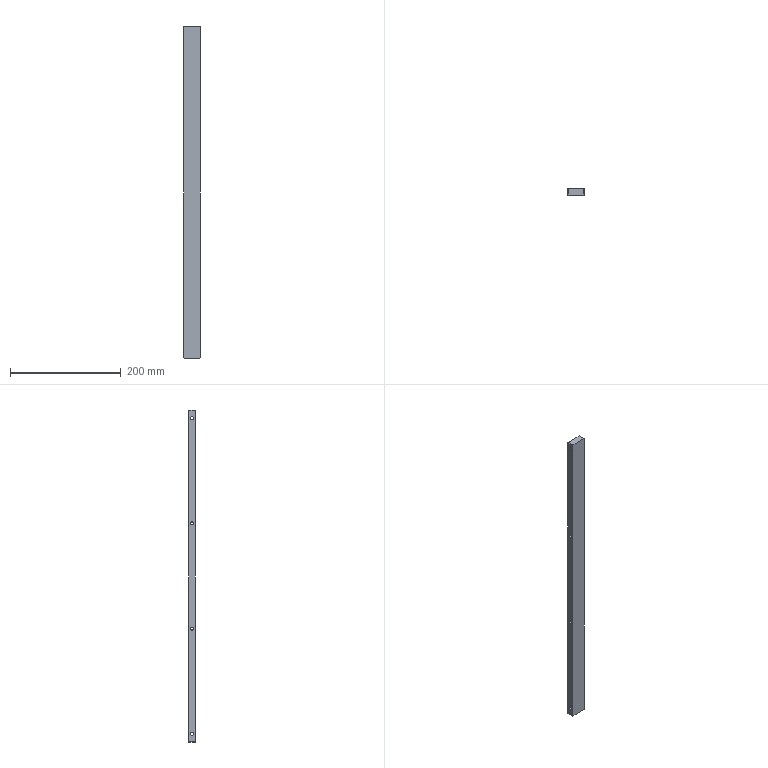Part | NX | features BREP 1 | 1 solid | 30 faces | box 30 x 12 x 600 mm | volume 212029 mm3 | cylinder 16 | plane 14 | commonest cylinder face diameters 5.5 x8 10 x8
STEP:
#1=CARTESIAN_POINT('',(10.,0.,20.));
#2=VERTEX_POINT('',#1);
#3=CARTESIAN_POINT('',(10.,0.,10.));
#4=VERTEX_POINT('',#3);
#5=CARTESIAN_POINT('',(10.,0.,15.));
#6=DIRECTION('',(1.,0.,0.));
#7=DIRECTION('',(0.,0.,-1.));
#8=AXIS2_PLACEMENT_3D('',#5,#6,#7);
#9=CIRCLE('',#8,5.);
#10=EDGE_CURVE('',#2,#4,#9,.T.);
#11=ORIENTED_EDGE('',*,*,#10,.F.);
#12=CARTESIAN_POINT('',(15.,0.,20.));
#13=VERTEX_POINT('',#12);
#14=CARTESIAN_POINT('',(15.,0.,20.));
#15=DIRECTION('',(1.,0.,0.));
#16=VECTOR('',#15,1000.);
#17=LINE('',#14,#16);
#18=EDGE_CURVE('',#2,#13,#17,.T.);
#19=ORIENTED_EDGE('',*,*,#18,.T.);
#20=CARTESIAN_POINT('',(15.,0.,10.));
#21=VERTEX_POINT('',#20);
#22=CARTESIAN_POINT('',(15.,0.,15.));
#23=DIRECTION('',(1.,0.,0.));
#24=DIRECTION('',(0.,0.,-1.));
#25=AXIS2_PLACEMENT_3D('',#22,#23,#24);
#26=CIRCLE('',#25,5.);
#27=EDGE_CURVE('',#13,#21,#26,.T.);
#28=ORIENTED_EDGE('',*,*,#27,.T.);
#29=CARTESIAN_POINT('',(15.,0.,10.));
#30=DIRECTION('',(1.,0.,0.));
#31=VECTOR('',#30,1000.);
#32=LINE('',#29,#31);
#33=EDGE_CURVE('',#4,#21,#32,.T.);
#34=ORIENTED_EDGE('',*,*,#33,.F.);
#35=EDGE_LOOP('',(#11,#19,#28,#34));
#36=FACE_BOUND('',#35,.T.);
#37=CARTESIAN_POINT('',(15.,0.,15.));
#38=DIRECTION('',(1.,0.,0.));
#39=DIRECTION('',(0.,0.,-1.));
#40=AXIS2_PLACEMENT_3D('',#37,#38,#39);
#41=CYLINDRICAL_SURFACE('',#40,5.);
#42=ADVANCED_FACE('',(#36),#41,.F.);
#43=CARTESIAN_POINT('',(-15.,0.,17.75));
#44=VERTEX_POINT('',#43);
#45=CARTESIAN_POINT('',(-15.,0.,12.25));
#46=VERTEX_POINT('',#45);
#47=CARTESIAN_POINT('',(-15.,0.,15.));
#48=DIRECTION('',(1.,0.,0.));
#49=DIRECTION('',(0.,0.,-1.));
#50=AXIS2_PLACEMENT_3D('',#47,#48,#49);
#51=CIRCLE('',#50,2.75);
#52=EDGE_CURVE('',#44,#46,#51,.T.);
#53=ORIENTED_EDGE('',*,*,#52,.F.);
#54=CARTESIAN_POINT('',(10.,0.,17.75));
#55=VERTEX_POINT('',#54);
#56=CARTESIAN_POINT('',(15.,0.,17.75));
#57=DIRECTION('',(1.,0.,0.));
#58=VECTOR('',#57,1000.);
#59=LINE('',#56,#58);
#60=EDGE_CURVE('',#44,#55,#59,.T.);
#61=ORIENTED_EDGE('',*,*,#60,.T.);
#62=CARTESIAN_POINT('',(10.,0.,12.25));
#63=VERTEX_POINT('',#62);
#64=CARTESIAN_POINT('',(10.,0.,15.));
#65=DIRECTION('',(1.,0.,0.));
#66=DIRECTION('',(0.,0.,-1.));
#67=AXIS2_PLACEMENT_3D('',#64,#65,#66);
#68=CIRCLE('',#67,2.75);
#69=EDGE_CURVE('',#55,#63,#68,.T.);
#70=ORIENTED_EDGE('',*,*,#69,.T.);
#71=CARTESIAN_POINT('',(15.,0.,12.25));
#72=DIRECTION('',(1.,0.,0.));
#73=VECTOR('',#72,1000.);
#74=LINE('',#71,#73);
#75=EDGE_CURVE('',#46,#63,#74,.T.);
#76=ORIENTED_EDGE('',*,*,#75,.F.);
#77=EDGE_LOOP('',(#53,#61,#70,#76));
#78=FACE_BOUND('',#77,.T.);
#79=CARTESIAN_POINT('',(15.,0.,15.));
#80=DIRECTION('',(1.,0.,0.));
#81=DIRECTION('',(0.,0.,-1.));
#82=AXIS2_PLACEMENT_3D('',#79,#80,#81);
#83=CYLINDRICAL_SURFACE('',#82,2.75);
#84=ADVANCED_FACE('',(#78),#83,.F.);
#85=CARTESIAN_POINT('',(10.,0.,210.));
#86=VERTEX_POINT('',#85);
#87=CARTESIAN_POINT('',(10.,0.,200.));
#88=VERTEX_POINT('',#87);
#89=CARTESIAN_POINT('',(10.,0.,205.));
#90=DIRECTION('',(1.,0.,0.));
#91=DIRECTION('',(0.,0.,-1.));
#92=AXIS2_PLACEMENT_3D('',#89,#90,#91);
#93=CIRCLE('',#92,5.);
#94=EDGE_CURVE('',#86,#88,#93,.T.);
#95=ORIENTED_EDGE('',*,*,#94,.F.);
#96=CARTESIAN_POINT('',(15.,0.,210.));
#97=VERTEX_POINT('',#96);
#98=CARTESIAN_POINT('',(15.,0.,210.));
#99=DIRECTION('',(1.,0.,0.));
#100=VECTOR('',#99,1000.);
#101=LINE('',#98,#100);
#102=EDGE_CURVE('',#86,#97,#101,.T.);
#103=ORIENTED_EDGE('',*,*,#102,.T.);
#104=CARTESIAN_POINT('',(15.,0.,200.));
#105=VERTEX_POINT('',#104);
#106=CARTESIAN_POINT('',(15.,0.,205.));
#107=DIRECTION('',(1.,0.,0.));
#108=DIRECTION('',(0.,0.,-1.));
#109=AXIS2_PLACEMENT_3D('',#106,#107,#108);
#110=CIRCLE('',#109,5.);
#111=EDGE_CURVE('',#97,#105,#110,.T.);
#112=ORIENTED_EDGE('',*,*,#111,.T.);
#113=CARTESIAN_POINT('',(15.,0.,200.));
#114=DIRECTION('',(1.,0.,0.));
#115=VECTOR('',#114,1000.);
#116=LINE('',#113,#115);
#117=EDGE_CURVE('',#88,#105,#116,.T.);
#118=ORIENTED_EDGE('',*,*,#117,.F.);
#119=EDGE_LOOP('',(#95,#103,#112,#118));
#120=FACE_BOUND('',#119,.T.);
#121=CARTESIAN_POINT('',(15.,0.,205.));
#122=DIRECTION('',(1.,0.,0.));
#123=DIRECTION('',(0.,0.,-1.));
#124=AXIS2_PLACEMENT_3D('',#121,#122,#123);
#125=CYLINDRICAL_SURFACE('',#124,5.);
#126=ADVANCED_FACE('',(#120),#125,.F.);
#127=CARTESIAN_POINT('',(-15.,0.,207.75));
#128=VERTEX_POINT('',#127);
#129=CARTESIAN_POINT('',(-15.,0.,202.25));
#130=VERTEX_POINT('',#129);
#131=CARTESIAN_POINT('',(-15.,0.,205.));
#132=DIRECTION('',(1.,0.,0.));
#133=DIRECTION('',(0.,0.,-1.));
#134=AXIS2_PLACEMENT_3D('',#131,#132,#133);
#135=CIRCLE('',#134,2.75);
#136=EDGE_CURVE('',#128,#130,#135,.T.);
#137=ORIENTED_EDGE('',*,*,#136,.F.);
#138=CARTESIAN_POINT('',(10.,0.,207.75));
#139=VERTEX_POINT('',#138);
#140=CARTESIAN_POINT('',(15.,0.,207.75));
#141=DIRECTION('',(1.,0.,0.));
#142=VECTOR('',#141,1000.);
#143=LINE('',#140,#142);
#144=EDGE_CURVE('',#128,#139,#143,.T.);
#145=ORIENTED_EDGE('',*,*,#144,.T.);
#146=CARTESIAN_POINT('',(10.,0.,202.25));
#147=VERTEX_POINT('',#146);
#148=CARTESIAN_POINT('',(10.,0.,205.));
#149=DIRECTION('',(1.,0.,0.));
#150=DIRECTION('',(0.,0.,-1.));
#151=AXIS2_PLACEMENT_3D('',#148,#149,#150);
#152=CIRCLE('',#151,2.75);
#153=EDGE_CURVE('',#139,#147,#152,.T.);
#154=ORIENTED_EDGE('',*,*,#153,.T.);
#155=CARTESIAN_POINT('',(15.,0.,202.25));
#156=DIRECTION('',(1.,0.,0.));
#157=VECTOR('',#156,1000.);
#158=LINE('',#155,#157);
#159=EDGE_CURVE('',#130,#147,#158,.T.);
#160=ORIENTED_EDGE('',*,*,#159,.F.);
#161=EDGE_LOOP('',(#137,#145,#154,#160));
#162=FACE_BOUND('',#161,.T.);
#163=CARTESIAN_POINT('',(15.,0.,205.));
#164=DIRECTION('',(1.,0.,0.));
#165=DIRECTION('',(0.,0.,-1.));
#166=AXIS2_PLACEMENT_3D('',#163,#164,#165);
#167=CYLINDRICAL_SURFACE('',#166,2.75);
#168=ADVANCED_FACE('',(#162),#167,.F.);
#169=CARTESIAN_POINT('',(10.,0.,400.));
#170=VERTEX_POINT('',#169);
#171=CARTESIAN_POINT('',(10.,0.,390.));
#172=VERTEX_POINT('',#171);
#173=CARTESIAN_POINT('',(10.,0.,395.));
#174=DIRECTION('',(1.,0.,0.));
#175=DIRECTION('',(0.,0.,-1.));
#176=AXIS2_PLACEMENT_3D('',#173,#174,#175);
#177=CIRCLE('',#176,5.);
#178=EDGE_CURVE('',#170,#172,#177,.T.);
#179=ORIENTED_EDGE('',*,*,#178,.F.);
#180=CARTESIAN_POINT('',(15.,0.,400.));
#181=VERTEX_POINT('',#180);
#182=CARTESIAN_POINT('',(15.,0.,400.));
#183=DIRECTION('',(1.,0.,0.));
#184=VECTOR('',#183,1000.);
#185=LINE('',#182,#184);
#186=EDGE_CURVE('',#170,#181,#185,.T.);
#187=ORIENTED_EDGE('',*,*,#186,.T.);
#188=CARTESIAN_POINT('',(15.,0.,390.));
#189=VERTEX_POINT('',#188);
#190=CARTESIAN_POINT('',(15.,0.,395.));
#191=DIRECTION('',(1.,0.,0.));
#192=DIRECTION('',(0.,0.,-1.));
#193=AXIS2_PLACEMENT_3D('',#190,#191,#192);
#194=CIRCLE('',#193,5.);
#195=EDGE_CURVE('',#181,#189,#194,.T.);
#196=ORIENTED_EDGE('',*,*,#195,.T.);
#197=CARTESIAN_POINT('',(15.,0.,390.));
#198=DIRECTION('',(1.,0.,0.));
#199=VECTOR('',#198,1000.);
#200=LINE('',#197,#199);
#201=EDGE_CURVE('',#172,#189,#200,.T.);
#202=ORIENTED_EDGE('',*,*,#201,.F.);
#203=EDGE_LOOP('',(#179,#187,#196,#202));
#204=FACE_BOUND('',#203,.T.);
#205=CARTESIAN_POINT('',(15.,0.,395.));
#206=DIRECTION('',(1.,0.,0.));
#207=DIRECTION('',(0.,0.,-1.));
#208=AXIS2_PLACEMENT_3D('',#205,#206,#207);
#209=CYLINDRICAL_SURFACE('',#208,5.);
#210=ADVANCED_FACE('',(#204),#209,.F.);
#211=CARTESIAN_POINT('',(-15.,0.,397.75));
#212=VERTEX_POINT('',#211);
#213=CARTESIAN_POINT('',(-15.,0.,392.25));
#214=VERTEX_POINT('',#213);
#215=CARTESIAN_POINT('',(-15.,0.,395.));
#216=DIRECTION('',(1.,0.,0.));
#217=DIRECTION('',(0.,0.,-1.));
#218=AXIS2_PLACEMENT_3D('',#215,#216,#217);
#219=CIRCLE('',#218,2.75);
#220=EDGE_CURVE('',#212,#214,#219,.T.);
#221=ORIENTED_EDGE('',*,*,#220,.F.);
#222=CARTESIAN_POINT('',(10.,0.,397.75));
#223=VERTEX_POINT('',#222);
#224=CARTESIAN_POINT('',(15.,0.,397.75));
#225=DIRECTION('',(1.,0.,0.));
#226=VECTOR('',#225,1000.);
#227=LINE('',#224,#226);
#228=EDGE_CURVE('',#212,#223,#227,.T.);
#229=ORIENTED_EDGE('',*,*,#228,.T.);
#230=CARTESIAN_POINT('',(10.,0.,392.25));
#231=VERTEX_POINT('',#230);
#232=CARTESIAN_POINT('',(10.,0.,395.));
#233=DIRECTION('',(1.,0.,0.));
#234=DIRECTION('',(0.,0.,-1.));
#235=AXIS2_PLACEMENT_3D('',#232,#233,#234);
#236=CIRCLE('',#235,2.75);
#237=EDGE_CURVE('',#223,#231,#236,.T.);
#238=ORIENTED_EDGE('',*,*,#237,.T.);
#239=CARTESIAN_POINT('',(15.,0.,392.25));
#240=DIRECTION('',(1.,0.,0.));
#241=VECTOR('',#240,1000.);
#242=LINE('',#239,#241);
#243=EDGE_CURVE('',#214,#231,#242,.T.);
#244=ORIENTED_EDGE('',*,*,#243,.F.);
#245=EDGE_LOOP('',(#221,#229,#238,#244));
#246=FACE_BOUND('',#245,.T.);
#247=CARTESIAN_POINT('',(15.,0.,395.));
#248=DIRECTION('',(1.,0.,0.));
#249=DIRECTION('',(0.,0.,-1.));
#250=AXIS2_PLACEMENT_3D('',#247,#248,#249);
#251=CYLINDRICAL_SURFACE('',#250,2.75);
#252=ADVANCED_FACE('',(#246),#251,.F.);
#253=CARTESIAN_POINT('',(10.,0.,590.));
#254=VERTEX_POINT('',#253);
#255=CARTESIAN_POINT('',(10.,0.,580.));
#256=VERTEX_POINT('',#255);
#257=CARTESIAN_POINT('',(10.,0.,585.));
#258=DIRECTION('',(1.,0.,0.));
#259=DIRECTION('',(0.,0.,-1.));
#260=AXIS2_PLACEMENT_3D('',#257,#258,#259);
#261=CIRCLE('',#260,5.);
#262=EDGE_CURVE('',#254,#256,#261,.T.);
#263=ORIENTED_EDGE('',*,*,#262,.F.);
#264=CARTESIAN_POINT('',(15.,0.,590.));
#265=VERTEX_POINT('',#264);
#266=CARTESIAN_POINT('',(15.,0.,590.));
#267=DIRECTION('',(1.,0.,0.));
#268=VECTOR('',#267,1000.);
#269=LINE('',#266,#268);
#270=EDGE_CURVE('',#254,#265,#269,.T.);
#271=ORIENTED_EDGE('',*,*,#270,.T.);
#272=CARTESIAN_POINT('',(15.,0.,580.));
#273=VERTEX_POINT('',#272);
#274=CARTESIAN_POINT('',(15.,0.,585.));
#275=DIRECTION('',(1.,0.,0.));
#276=DIRECTION('',(0.,0.,-1.));
#277=AXIS2_PLACEMENT_3D('',#274,#275,#276);
#278=CIRCLE('',#277,5.);
#279=EDGE_CURVE('',#265,#273,#278,.T.);
#280=ORIENTED_EDGE('',*,*,#279,.T.);
#281=CARTESIAN_POINT('',(15.,0.,580.));
#282=DIRECTION('',(1.,0.,0.));
#283=VECTOR('',#282,1000.);
#284=LINE('',#281,#283);
#285=EDGE_CURVE('',#256,#273,#284,.T.);
#286=ORIENTED_EDGE('',*,*,#285,.F.);
#287=EDGE_LOOP('',(#263,#271,#280,#286));
#288=FACE_BOUND('',#287,.T.);
#289=CARTESIAN_POINT('',(15.,0.,585.));
#290=DIRECTION('',(1.,0.,0.));
#291=DIRECTION('',(0.,0.,-1.));
#292=AXIS2_PLACEMENT_3D('',#289,#290,#291);
#293=CYLINDRICAL_SURFACE('',#292,5.);
#294=ADVANCED_FACE('',(#288),#293,.F.);
#295=CARTESIAN_POINT('',(-15.,0.,587.75));
#296=VERTEX_POINT('',#295);
#297=CARTESIAN_POINT('',(-15.,0.,582.25));
#298=VERTEX_POINT('',#297);
#299=CARTESIAN_POINT('',(-15.,0.,585.));
#300=DIRECTION('',(1.,0.,0.));
#301=DIRECTION('',(0.,0.,-1.));
#302=AXIS2_PLACEMENT_3D('',#299,#300,#301);
#303=CIRCLE('',#302,2.75);
#304=EDGE_CURVE('',#296,#298,#303,.T.);
#305=ORIENTED_EDGE('',*,*,#304,.F.);
#306=CARTESIAN_POINT('',(10.,0.,587.75));
#307=VERTEX_POINT('',#306);
#308=CARTESIAN_POINT('',(15.,0.,587.75));
#309=DIRECTION('',(1.,0.,0.));
#310=VECTOR('',#309,1000.);
#311=LINE('',#308,#310);
#312=EDGE_CURVE('',#296,#307,#311,.T.);
#313=ORIENTED_EDGE('',*,*,#312,.T.);
#314=CARTESIAN_POINT('',(10.,0.,582.25));
#315=VERTEX_POINT('',#314);
#316=CARTESIAN_POINT('',(10.,0.,585.));
#317=DIRECTION('',(1.,0.,0.));
#318=DIRECTION('',(0.,0.,-1.));
#319=AXIS2_PLACEMENT_3D('',#316,#317,#318);
#320=CIRCLE('',#319,2.75);
#321=EDGE_CURVE('',#307,#315,#320,.T.);
#322=ORIENTED_EDGE('',*,*,#321,.T.);
#323=CARTESIAN_POINT('',(15.,0.,582.25));
#324=DIRECTION('',(1.,0.,0.));
#325=VECTOR('',#324,1000.);
#326=LINE('',#323,#325);
#327=EDGE_CURVE('',#298,#315,#326,.T.);
#328=ORIENTED_EDGE('',*,*,#327,.F.);
#329=EDGE_LOOP('',(#305,#313,#322,#328));
#330=FACE_BOUND('',#329,.T.);
#331=CARTESIAN_POINT('',(15.,0.,585.));
#332=DIRECTION('',(1.,0.,0.));
#333=DIRECTION('',(0.,0.,-1.));
#334=AXIS2_PLACEMENT_3D('',#331,#332,#333);
#335=CYLINDRICAL_SURFACE('',#334,2.75);
#336=ADVANCED_FACE('',(#330),#335,.F.);
#337=CARTESIAN_POINT('',(15.,-6.,599.));
#338=VERTEX_POINT('',#337);
#339=CARTESIAN_POINT('',(15.,-6.,1.));
#340=VERTEX_POINT('',#339);
#341=CARTESIAN_POINT('',(15.,-6.,600.));
#342=DIRECTION('',(0.,0.,-1.));
#343=VECTOR('',#342,1000.);
#344=LINE('',#341,#343);
#345=EDGE_CURVE('',#338,#340,#344,.T.);
#346=ORIENTED_EDGE('',*,*,#345,.T.);
#347=CARTESIAN_POINT('',(15.,6.,1.));
#348=VERTEX_POINT('',#347);
#349=CARTESIAN_POINT('',(15.,6.,1.));
#350=DIRECTION('',(0.,1.,0.));
#351=VECTOR('',#350,1000.);
#352=LINE('',#349,#351);
#353=EDGE_CURVE('',#340,#348,#352,.T.);
#354=ORIENTED_EDGE('',*,*,#353,.T.);
#355=CARTESIAN_POINT('',(15.,6.,599.));
#356=VERTEX_POINT('',#355);
#357=CARTESIAN_POINT('',(15.,6.,600.));
#358=DIRECTION('',(0.,0.,-1.));
#359=VECTOR('',#358,1000.);
#360=LINE('',#357,#359);
#361=EDGE_CURVE('',#356,#348,#360,.T.);
#362=ORIENTED_EDGE('',*,*,#361,.F.);
#363=CARTESIAN_POINT('',(15.,-6.,599.));
#364=DIRECTION('',(0.,-1.,0.));
#365=VECTOR('',#364,1000.);
#366=LINE('',#363,#365);
#367=EDGE_CURVE('',#356,#338,#366,.T.);
#368=ORIENTED_EDGE('',*,*,#367,.T.);
#369=EDGE_LOOP('',(#346,#354,#362,#368));
#370=FACE_BOUND('',#369,.T.);
#371=CARTESIAN_POINT('',(15.,0.,15.));
#372=DIRECTION('',(1.,0.,0.));
#373=DIRECTION('',(0.,0.,-1.));
#374=AXIS2_PLACEMENT_3D('',#371,#372,#373);
#375=CIRCLE('',#374,5.);
#376=EDGE_CURVE('',#21,#13,#375,.T.);
#377=ORIENTED_EDGE('',*,*,#376,.F.);
#378=ORIENTED_EDGE('',*,*,#27,.F.);
#379=EDGE_LOOP('',(#377,#378));
#380=FACE_BOUND('',#379,.T.);
#381=CARTESIAN_POINT('',(15.,0.,205.));
#382=DIRECTION('',(1.,0.,0.));
#383=DIRECTION('',(0.,0.,-1.));
#384=AXIS2_PLACEMENT_3D('',#381,#382,#383);
#385=CIRCLE('',#384,5.);
#386=EDGE_CURVE('',#105,#97,#385,.T.);
#387=ORIENTED_EDGE('',*,*,#386,.F.);
#388=ORIENTED_EDGE('',*,*,#111,.F.);
#389=EDGE_LOOP('',(#387,#388));
#390=FACE_BOUND('',#389,.T.);
#391=CARTESIAN_POINT('',(15.,0.,395.));
#392=DIRECTION('',(1.,0.,0.));
#393=DIRECTION('',(0.,0.,-1.));
#394=AXIS2_PLACEMENT_3D('',#391,#392,#393);
#395=CIRCLE('',#394,5.);
#396=EDGE_CURVE('',#189,#181,#395,.T.);
#397=ORIENTED_EDGE('',*,*,#396,.F.);
#398=ORIENTED_EDGE('',*,*,#195,.F.);
#399=EDGE_LOOP('',(#397,#398));
#400=FACE_BOUND('',#399,.T.);
#401=CARTESIAN_POINT('',(15.,0.,585.));
#402=DIRECTION('',(1.,0.,0.));
#403=DIRECTION('',(0.,0.,-1.));
#404=AXIS2_PLACEMENT_3D('',#401,#402,#403);
#405=CIRCLE('',#404,5.);
#406=EDGE_CURVE('',#273,#265,#405,.T.);
#407=ORIENTED_EDGE('',*,*,#406,.F.);
#408=ORIENTED_EDGE('',*,*,#279,.F.);
#409=EDGE_LOOP('',(#407,#408));
#410=FACE_BOUND('',#409,.T.);
#411=CARTESIAN_POINT('',(15.,6.,600.));
#412=DIRECTION('',(-1.,0.,0.));
#413=DIRECTION('',(0.,1.,0.));
#414=AXIS2_PLACEMENT_3D('',#411,#412,#413);
#415=PLANE('',#414);
#416=ADVANCED_FACE('',(#370,#380,#390,#400,#410),#415,.F.);
#417=ORIENTED_EDGE('',*,*,#361,.T.);
#418=CARTESIAN_POINT('',(14.,6.,0.));
#419=VERTEX_POINT('',#418);
#420=CARTESIAN_POINT('',(15.,6.,1.));
#421=DIRECTION('',(-0.7071,0.,-0.7071));
#422=VECTOR('',#421,1000.);
#423=LINE('',#420,#422);
#424=EDGE_CURVE('',#348,#419,#423,.T.);
#425=ORIENTED_EDGE('',*,*,#424,.T.);
#426=CARTESIAN_POINT('',(-14.,6.,0.));
#427=VERTEX_POINT('',#426);
#428=CARTESIAN_POINT('',(-15.,6.,0.));
#429=DIRECTION('',(-1.,0.,0.));
#430=VECTOR('',#429,1000.);
#431=LINE('',#428,#430);
#432=EDGE_CURVE('',#419,#427,#431,.T.);
#433=ORIENTED_EDGE('',*,*,#432,.T.);
#434=CARTESIAN_POINT('',(-15.,6.,1.));
#435=VERTEX_POINT('',#434);
#436=CARTESIAN_POINT('',(-15.,6.,1.));
#437=DIRECTION('',(-0.7071,0.,0.7071));
#438=VECTOR('',#437,1000.);
#439=LINE('',#436,#438);
#440=EDGE_CURVE('',#427,#435,#439,.T.);
#441=ORIENTED_EDGE('',*,*,#440,.T.);
#442=CARTESIAN_POINT('',(-15.,6.,599.));
#443=VERTEX_POINT('',#442);
#444=CARTESIAN_POINT('',(-15.,6.,600.));
#445=DIRECTION('',(0.,0.,-1.));
#446=VECTOR('',#445,1000.);
#447=LINE('',#444,#446);
#448=EDGE_CURVE('',#443,#435,#447,.T.);
#449=ORIENTED_EDGE('',*,*,#448,.F.);
#450=CARTESIAN_POINT('',(-14.,6.,600.));
#451=VERTEX_POINT('',#450);
#452=CARTESIAN_POINT('',(-14.,6.,600.));
#453=DIRECTION('',(0.7071,0.,0.7071));
#454=VECTOR('',#453,1000.);
#455=LINE('',#452,#454);
#456=EDGE_CURVE('',#443,#451,#455,.T.);
#457=ORIENTED_EDGE('',*,*,#456,.T.);
#458=CARTESIAN_POINT('',(14.,6.,600.));
#459=VERTEX_POINT('',#458);
#460=CARTESIAN_POINT('',(-15.,6.,600.));
#461=DIRECTION('',(-1.,0.,0.));
#462=VECTOR('',#461,1000.);
#463=LINE('',#460,#462);
#464=EDGE_CURVE('',#459,#451,#463,.T.);
#465=ORIENTED_EDGE('',*,*,#464,.F.);
#466=CARTESIAN_POINT('',(14.,6.,600.));
#467=DIRECTION('',(0.7071,0.,-0.7071));
#468=VECTOR('',#467,1000.);
#469=LINE('',#466,#468);
#470=EDGE_CURVE('',#459,#356,#469,.T.);
#471=ORIENTED_EDGE('',*,*,#470,.T.);
#472=EDGE_LOOP('',(#417,#425,#433,#441,#449,#457,#465,#471));
#473=FACE_BOUND('',#472,.T.);
#474=CARTESIAN_POINT('',(-15.,6.,600.));
#475=DIRECTION('',(0.,-1.,0.));
#476=DIRECTION('',(0.,0.,-1.));
#477=AXIS2_PLACEMENT_3D('',#474,#475,#476);
#478=PLANE('',#477);
#479=ADVANCED_FACE('',(#473),#478,.F.);
#480=ORIENTED_EDGE('',*,*,#448,.T.);
#481=CARTESIAN_POINT('',(-15.,-6.,1.));
#482=VERTEX_POINT('',#481);
#483=CARTESIAN_POINT('',(-15.,6.,1.));
#484=DIRECTION('',(0.,-1.,0.));
#485=VECTOR('',#484,1000.);
#486=LINE('',#483,#485);
#487=EDGE_CURVE('',#435,#482,#486,.T.);
#488=ORIENTED_EDGE('',*,*,#487,.T.);
#489=CARTESIAN_POINT('',(-15.,-6.,599.));
#490=VERTEX_POINT('',#489);
#491=CARTESIAN_POINT('',(-15.,-6.,600.));
#492=DIRECTION('',(0.,0.,-1.));
#493=VECTOR('',#492,1000.);
#494=LINE('',#491,#493);
#495=EDGE_CURVE('',#490,#482,#494,.T.);
#496=ORIENTED_EDGE('',*,*,#495,.F.);
#497=CARTESIAN_POINT('',(-15.,6.,599.));
#498=DIRECTION('',(0.,1.,0.));
#499=VECTOR('',#498,1000.);
#500=LINE('',#497,#499);
#501=EDGE_CURVE('',#490,#443,#500,.T.);
#502=ORIENTED_EDGE('',*,*,#501,.T.);
#503=EDGE_LOOP('',(#480,#488,#496,#502));
#504=FACE_BOUND('',#503,.T.);
#505=CARTESIAN_POINT('',(-15.,0.,15.));
#506=DIRECTION('',(1.,0.,0.));
#507=DIRECTION('',(0.,0.,-1.));
#508=AXIS2_PLACEMENT_3D('',#505,#506,#507);
#509=CIRCLE('',#508,2.75);
#510=EDGE_CURVE('',#46,#44,#509,.T.);
#511=ORIENTED_EDGE('',*,*,#510,.T.);
#512=ORIENTED_EDGE('',*,*,#52,.T.);
#513=EDGE_LOOP('',(#511,#512));
#514=FACE_BOUND('',#513,.T.);
#515=CARTESIAN_POINT('',(-15.,0.,205.));
#516=DIRECTION('',(1.,0.,0.));
#517=DIRECTION('',(0.,0.,-1.));
#518=AXIS2_PLACEMENT_3D('',#515,#516,#517);
#519=CIRCLE('',#518,2.75);
#520=EDGE_CURVE('',#130,#128,#519,.T.);
#521=ORIENTED_EDGE('',*,*,#520,.T.);
#522=ORIENTED_EDGE('',*,*,#136,.T.);
#523=EDGE_LOOP('',(#521,#522));
#524=FACE_BOUND('',#523,.T.);
#525=CARTESIAN_POINT('',(-15.,0.,395.));
#526=DIRECTION('',(1.,0.,0.));
#527=DIRECTION('',(0.,0.,-1.));
#528=AXIS2_PLACEMENT_3D('',#525,#526,#527);
#529=CIRCLE('',#528,2.75);
#530=EDGE_CURVE('',#214,#212,#529,.T.);
#531=ORIENTED_EDGE('',*,*,#530,.T.);
#532=ORIENTED_EDGE('',*,*,#220,.T.);
#533=EDGE_LOOP('',(#531,#532));
#534=FACE_BOUND('',#533,.T.);
#535=CARTESIAN_POINT('',(-15.,0.,585.));
#536=DIRECTION('',(1.,0.,0.));
#537=DIRECTION('',(0.,0.,-1.));
#538=AXIS2_PLACEMENT_3D('',#535,#536,#537);
#539=CIRCLE('',#538,2.75);
#540=EDGE_CURVE('',#298,#296,#539,.T.);
#541=ORIENTED_EDGE('',*,*,#540,.T.);
#542=ORIENTED_EDGE('',*,*,#304,.T.);
#543=EDGE_LOOP('',(#541,#542));
#544=FACE_BOUND('',#543,.T.);
#545=CARTESIAN_POINT('',(-15.,6.,600.));
#546=DIRECTION('',(1.,0.,0.));
#547=DIRECTION('',(0.,1.,0.));
#548=AXIS2_PLACEMENT_3D('',#545,#546,#547);
#549=PLANE('',#548);
#550=ADVANCED_FACE('',(#504,#514,#524,#534,#544),#549,.F.);
#551=CARTESIAN_POINT('',(-14.,-6.,0.));
#552=VERTEX_POINT('',#551);
#553=CARTESIAN_POINT('',(14.,-6.,0.));
#554=VERTEX_POINT('',#553);
#555=CARTESIAN_POINT('',(-15.,-6.,0.));
#556=DIRECTION('',(1.,0.,0.));
#557=VECTOR('',#556,1000.);
#558=LINE('',#555,#557);
#559=EDGE_CURVE('',#552,#554,#558,.T.);
#560=ORIENTED_EDGE('',*,*,#559,.T.);
#561=CARTESIAN_POINT('',(15.,-6.,1.));
#562=DIRECTION('',(0.7071,0.,0.7071));
#563=VECTOR('',#562,1000.);
#564=LINE('',#561,#563);
#565=EDGE_CURVE('',#554,#340,#564,.T.);
#566=ORIENTED_EDGE('',*,*,#565,.T.);
#567=ORIENTED_EDGE('',*,*,#345,.F.);
#568=CARTESIAN_POINT('',(14.,-6.,600.));
#569=VERTEX_POINT('',#568);
#570=CARTESIAN_POINT('',(14.,-6.,600.));
#571=DIRECTION('',(-0.7071,0.,0.7071));
#572=VECTOR('',#571,1000.);
#573=LINE('',#570,#572);
#574=EDGE_CURVE('',#338,#569,#573,.T.);
#575=ORIENTED_EDGE('',*,*,#574,.T.);
#576=CARTESIAN_POINT('',(-14.,-6.,600.));
#577=VERTEX_POINT('',#576);
#578=CARTESIAN_POINT('',(-15.,-6.,600.));
#579=DIRECTION('',(1.,0.,0.));
#580=VECTOR('',#579,1000.);
#581=LINE('',#578,#580);
#582=EDGE_CURVE('',#577,#569,#581,.T.);
#583=ORIENTED_EDGE('',*,*,#582,.F.);
#584=CARTESIAN_POINT('',(-14.,-6.,600.));
#585=DIRECTION('',(-0.7071,0.,-0.7071));
#586=VECTOR('',#585,1000.);
#587=LINE('',#584,#586);
#588=EDGE_CURVE('',#577,#490,#587,.T.);
#589=ORIENTED_EDGE('',*,*,#588,.T.);
#590=ORIENTED_EDGE('',*,*,#495,.T.);
#591=CARTESIAN_POINT('',(-15.,-6.,1.));
#592=DIRECTION('',(0.7071,0.,-0.7071));
#593=VECTOR('',#592,1000.);
#594=LINE('',#591,#593);
#595=EDGE_CURVE('',#482,#552,#594,.T.);
#596=ORIENTED_EDGE('',*,*,#595,.T.);
#597=EDGE_LOOP('',(#560,#566,#567,#575,#583,#589,#590,#596));
#598=FACE_BOUND('',#597,.T.);
#599=CARTESIAN_POINT('',(-15.,-6.,600.));
#600=DIRECTION('',(0.,1.,0.));
#601=DIRECTION('',(1.,0.,0.));
#602=AXIS2_PLACEMENT_3D('',#599,#600,#601);
#603=PLANE('',#602);
#604=ADVANCED_FACE('',(#598),#603,.F.);
#605=ORIENTED_EDGE('',*,*,#582,.T.);
#606=CARTESIAN_POINT('',(14.,6.,600.));
#607=DIRECTION('',(0.,1.,0.));
#608=VECTOR('',#607,1000.);
#609=LINE('',#606,#608);
#610=EDGE_CURVE('',#569,#459,#609,.T.);
#611=ORIENTED_EDGE('',*,*,#610,.T.);
#612=ORIENTED_EDGE('',*,*,#464,.T.);
#613=CARTESIAN_POINT('',(-14.,-6.,600.));
#614=DIRECTION('',(0.,-1.,0.));
#615=VECTOR('',#614,1000.);
#616=LINE('',#613,#615);
#617=EDGE_CURVE('',#451,#577,#616,.T.);
#618=ORIENTED_EDGE('',*,*,#617,.T.);
#619=EDGE_LOOP('',(#605,#611,#612,#618));
#620=FACE_BOUND('',#619,.T.);
#621=CARTESIAN_POINT('',(15.,-6.,600.));
#622=DIRECTION('',(0.,0.,1.));
#623=DIRECTION('',(1.,0.,0.));
#624=AXIS2_PLACEMENT_3D('',#621,#622,#623);
#625=PLANE('',#624);
#626=ADVANCED_FACE('',(#620),#625,.T.);
#627=ORIENTED_EDGE('',*,*,#432,.F.);
#628=CARTESIAN_POINT('',(14.,-6.,0.));
#629=DIRECTION('',(0.,-1.,0.));
#630=VECTOR('',#629,1000.);
#631=LINE('',#628,#630);
#632=EDGE_CURVE('',#419,#554,#631,.T.);
#633=ORIENTED_EDGE('',*,*,#632,.T.);
#634=ORIENTED_EDGE('',*,*,#559,.F.);
#635=CARTESIAN_POINT('',(-14.,-6.,0.));
#636=DIRECTION('',(0.,1.,0.));
#637=VECTOR('',#636,1000.);
#638=LINE('',#635,#637);
#639=EDGE_CURVE('',#552,#427,#638,.T.);
#640=ORIENTED_EDGE('',*,*,#639,.T.);
#641=EDGE_LOOP('',(#627,#633,#634,#640));
#642=FACE_BOUND('',#641,.T.);
#643=CARTESIAN_POINT('',(15.,-6.,0.));
#644=DIRECTION('',(0.,0.,1.));
#645=DIRECTION('',(1.,0.,0.));
#646=AXIS2_PLACEMENT_3D('',#643,#644,#645);
#647=PLANE('',#646);
#648=ADVANCED_FACE('',(#642),#647,.F.);
#649=ORIENTED_EDGE('',*,*,#312,.F.);
#650=ORIENTED_EDGE('',*,*,#540,.F.);
#651=ORIENTED_EDGE('',*,*,#327,.T.);
#652=CARTESIAN_POINT('',(10.,0.,585.));
#653=DIRECTION('',(1.,0.,0.));
#654=DIRECTION('',(0.,0.,-1.));
#655=AXIS2_PLACEMENT_3D('',#652,#653,#654);
#656=CIRCLE('',#655,2.75);
#657=EDGE_CURVE('',#315,#307,#656,.T.);
#658=ORIENTED_EDGE('',*,*,#657,.T.);
#659=EDGE_LOOP('',(#649,#650,#651,#658));
#660=FACE_BOUND('',#659,.T.);
#661=CARTESIAN_POINT('',(15.,0.,585.));
#662=DIRECTION('',(1.,0.,0.));
#663=DIRECTION('',(0.,0.,-1.));
#664=AXIS2_PLACEMENT_3D('',#661,#662,#663);
#665=CYLINDRICAL_SURFACE('',#664,2.75);
#666=ADVANCED_FACE('',(#660),#665,.F.);
#667=CARTESIAN_POINT('',(10.,0.,585.));
#668=DIRECTION('',(1.,0.,0.));
#669=DIRECTION('',(0.,0.,-1.));
#670=AXIS2_PLACEMENT_3D('',#667,#668,#669);
#671=CIRCLE('',#670,5.);
#672=EDGE_CURVE('',#256,#254,#671,.T.);
#673=ORIENTED_EDGE('',*,*,#672,.T.);
#674=ORIENTED_EDGE('',*,*,#262,.T.);
#675=EDGE_LOOP('',(#673,#674));
#676=FACE_BOUND('',#675,.T.);
#677=ORIENTED_EDGE('',*,*,#657,.F.);
#678=ORIENTED_EDGE('',*,*,#321,.F.);
#679=EDGE_LOOP('',(#677,#678));
#680=FACE_BOUND('',#679,.T.);
#681=CARTESIAN_POINT('',(10.,2.75,585.));
#682=DIRECTION('',(-1.,0.,0.));
#683=DIRECTION('',(0.,0.,1.));
#684=AXIS2_PLACEMENT_3D('',#681,#682,#683);
#685=PLANE('',#684);
#686=ADVANCED_FACE('',(#676,#680),#685,.F.);
#687=ORIENTED_EDGE('',*,*,#270,.F.);
#688=ORIENTED_EDGE('',*,*,#672,.F.);
#689=ORIENTED_EDGE('',*,*,#285,.T.);
#690=ORIENTED_EDGE('',*,*,#406,.T.);
#691=EDGE_LOOP('',(#687,#688,#689,#690));
#692=FACE_BOUND('',#691,.T.);
#693=CARTESIAN_POINT('',(15.,0.,585.));
#694=DIRECTION('',(1.,0.,0.));
#695=DIRECTION('',(0.,0.,-1.));
#696=AXIS2_PLACEMENT_3D('',#693,#694,#695);
#697=CYLINDRICAL_SURFACE('',#696,5.);
#698=ADVANCED_FACE('',(#692),#697,.F.);
#699=ORIENTED_EDGE('',*,*,#565,.F.);
#700=ORIENTED_EDGE('',*,*,#632,.F.);
#701=ORIENTED_EDGE('',*,*,#424,.F.);
#702=ORIENTED_EDGE('',*,*,#353,.F.);
#703=EDGE_LOOP('',(#699,#700,#701,#702));
#704=FACE_BOUND('',#703,.T.);
#705=CARTESIAN_POINT('',(15.,6.,1.));
#706=DIRECTION('',(-0.7071,0.,0.7071));
#707=DIRECTION('',(0.,1.,0.));
#708=AXIS2_PLACEMENT_3D('',#705,#706,#707);
#709=PLANE('',#708);
#710=ADVANCED_FACE('',(#704),#709,.F.);
#711=ORIENTED_EDGE('',*,*,#440,.F.);
#712=ORIENTED_EDGE('',*,*,#639,.F.);
#713=ORIENTED_EDGE('',*,*,#595,.F.);
#714=ORIENTED_EDGE('',*,*,#487,.F.);
#715=EDGE_LOOP('',(#711,#712,#713,#714));
#716=FACE_BOUND('',#715,.T.);
#717=CARTESIAN_POINT('',(-15.,6.,1.));
#718=DIRECTION('',(0.7071,0.,0.7071));
#719=DIRECTION('',(0.,-1.,0.));
#720=AXIS2_PLACEMENT_3D('',#717,#718,#719);
#721=PLANE('',#720);
#722=ADVANCED_FACE('',(#716),#721,.F.);
#723=ORIENTED_EDGE('',*,*,#574,.F.);
#724=ORIENTED_EDGE('',*,*,#367,.F.);
#725=ORIENTED_EDGE('',*,*,#470,.F.);
#726=ORIENTED_EDGE('',*,*,#610,.F.);
#727=EDGE_LOOP('',(#723,#724,#725,#726));
#728=FACE_BOUND('',#727,.T.);
#729=CARTESIAN_POINT('',(14.,-6.,600.));
#730=DIRECTION('',(0.7071,0.,0.7071));
#731=DIRECTION('',(0.,-1.,0.));
#732=AXIS2_PLACEMENT_3D('',#729,#730,#731);
#733=PLANE('',#732);
#734=ADVANCED_FACE('',(#728),#733,.T.);
#735=ORIENTED_EDGE('',*,*,#456,.F.);
#736=ORIENTED_EDGE('',*,*,#501,.F.);
#737=ORIENTED_EDGE('',*,*,#588,.F.);
#738=ORIENTED_EDGE('',*,*,#617,.F.);
#739=EDGE_LOOP('',(#735,#736,#737,#738));
#740=FACE_BOUND('',#739,.T.);
#741=CARTESIAN_POINT('',(-14.,-6.,600.));
#742=DIRECTION('',(-0.7071,0.,0.7071));
#743=DIRECTION('',(0.,1.,0.));
#744=AXIS2_PLACEMENT_3D('',#741,#742,#743);
#745=PLANE('',#744);
#746=ADVANCED_FACE('',(#740),#745,.T.);
#747=ORIENTED_EDGE('',*,*,#228,.F.);
#748=ORIENTED_EDGE('',*,*,#530,.F.);
#749=ORIENTED_EDGE('',*,*,#243,.T.);
#750=CARTESIAN_POINT('',(10.,0.,395.));
#751=DIRECTION('',(1.,0.,0.));
#752=DIRECTION('',(0.,0.,-1.));
#753=AXIS2_PLACEMENT_3D('',#750,#751,#752);
#754=CIRCLE('',#753,2.75);
#755=EDGE_CURVE('',#231,#223,#754,.T.);
#756=ORIENTED_EDGE('',*,*,#755,.T.);
#757=EDGE_LOOP('',(#747,#748,#749,#756));
#758=FACE_BOUND('',#757,.T.);
#759=CARTESIAN_POINT('',(15.,0.,395.));
#760=DIRECTION('',(1.,0.,0.));
#761=DIRECTION('',(0.,0.,-1.));
#762=AXIS2_PLACEMENT_3D('',#759,#760,#761);
#763=CYLINDRICAL_SURFACE('',#762,2.75);
#764=ADVANCED_FACE('',(#758),#763,.F.);
#765=CARTESIAN_POINT('',(10.,0.,395.));
#766=DIRECTION('',(1.,0.,0.));
#767=DIRECTION('',(0.,0.,-1.));
#768=AXIS2_PLACEMENT_3D('',#765,#766,#767);
#769=CIRCLE('',#768,5.);
#770=EDGE_CURVE('',#172,#170,#769,.T.);
#771=ORIENTED_EDGE('',*,*,#770,.T.);
#772=ORIENTED_EDGE('',*,*,#178,.T.);
#773=EDGE_LOOP('',(#771,#772));
#774=FACE_BOUND('',#773,.T.);
#775=ORIENTED_EDGE('',*,*,#755,.F.);
#776=ORIENTED_EDGE('',*,*,#237,.F.);
#777=EDGE_LOOP('',(#775,#776));
#778=FACE_BOUND('',#777,.T.);
#779=CARTESIAN_POINT('',(10.,2.75,395.));
#780=DIRECTION('',(-1.,0.,0.));
#781=DIRECTION('',(0.,0.,1.));
#782=AXIS2_PLACEMENT_3D('',#779,#780,#781);
#783=PLANE('',#782);
#784=ADVANCED_FACE('',(#774,#778),#783,.F.);
#785=ORIENTED_EDGE('',*,*,#186,.F.);
#786=ORIENTED_EDGE('',*,*,#770,.F.);
#787=ORIENTED_EDGE('',*,*,#201,.T.);
#788=ORIENTED_EDGE('',*,*,#396,.T.);
#789=EDGE_LOOP('',(#785,#786,#787,#788));
#790=FACE_BOUND('',#789,.T.);
#791=CARTESIAN_POINT('',(15.,0.,395.));
#792=DIRECTION('',(1.,0.,0.));
#793=DIRECTION('',(0.,0.,-1.));
#794=AXIS2_PLACEMENT_3D('',#791,#792,#793);
#795=CYLINDRICAL_SURFACE('',#794,5.);
#796=ADVANCED_FACE('',(#790),#795,.F.);
#797=ORIENTED_EDGE('',*,*,#144,.F.);
#798=ORIENTED_EDGE('',*,*,#520,.F.);
#799=ORIENTED_EDGE('',*,*,#159,.T.);
#800=CARTESIAN_POINT('',(10.,0.,205.));
#801=DIRECTION('',(1.,0.,0.));
#802=DIRECTION('',(0.,0.,-1.));
#803=AXIS2_PLACEMENT_3D('',#800,#801,#802);
#804=CIRCLE('',#803,2.75);
#805=EDGE_CURVE('',#147,#139,#804,.T.);
#806=ORIENTED_EDGE('',*,*,#805,.T.);
#807=EDGE_LOOP('',(#797,#798,#799,#806));
#808=FACE_BOUND('',#807,.T.);
#809=CARTESIAN_POINT('',(15.,0.,205.));
#810=DIRECTION('',(1.,0.,0.));
#811=DIRECTION('',(0.,0.,-1.));
#812=AXIS2_PLACEMENT_3D('',#809,#810,#811);
#813=CYLINDRICAL_SURFACE('',#812,2.75);
#814=ADVANCED_FACE('',(#808),#813,.F.);
#815=CARTESIAN_POINT('',(10.,0.,205.));
#816=DIRECTION('',(1.,0.,0.));
#817=DIRECTION('',(0.,0.,-1.));
#818=AXIS2_PLACEMENT_3D('',#815,#816,#817);
#819=CIRCLE('',#818,5.);
#820=EDGE_CURVE('',#88,#86,#819,.T.);
#821=ORIENTED_EDGE('',*,*,#820,.T.);
#822=ORIENTED_EDGE('',*,*,#94,.T.);
#823=EDGE_LOOP('',(#821,#822));
#824=FACE_BOUND('',#823,.T.);
#825=ORIENTED_EDGE('',*,*,#805,.F.);
#826=ORIENTED_EDGE('',*,*,#153,.F.);
#827=EDGE_LOOP('',(#825,#826));
#828=FACE_BOUND('',#827,.T.);
#829=CARTESIAN_POINT('',(10.,2.75,205.));
#830=DIRECTION('',(-1.,0.,0.));
#831=DIRECTION('',(0.,0.,1.));
#832=AXIS2_PLACEMENT_3D('',#829,#830,#831);
#833=PLANE('',#832);
#834=ADVANCED_FACE('',(#824,#828),#833,.F.);
#835=ORIENTED_EDGE('',*,*,#102,.F.);
#836=ORIENTED_EDGE('',*,*,#820,.F.);
#837=ORIENTED_EDGE('',*,*,#117,.T.);
#838=ORIENTED_EDGE('',*,*,#386,.T.);
#839=EDGE_LOOP('',(#835,#836,#837,#838));
#840=FACE_BOUND('',#839,.T.);
#841=CARTESIAN_POINT('',(15.,0.,205.));
#842=DIRECTION('',(1.,0.,0.));
#843=DIRECTION('',(0.,0.,-1.));
#844=AXIS2_PLACEMENT_3D('',#841,#842,#843);
#845=CYLINDRICAL_SURFACE('',#844,5.);
#846=ADVANCED_FACE('',(#840),#845,.F.);
#847=ORIENTED_EDGE('',*,*,#60,.F.);
#848=ORIENTED_EDGE('',*,*,#510,.F.);
#849=ORIENTED_EDGE('',*,*,#75,.T.);
#850=CARTESIAN_POINT('',(10.,0.,15.));
#851=DIRECTION('',(1.,0.,0.));
#852=DIRECTION('',(0.,0.,-1.));
#853=AXIS2_PLACEMENT_3D('',#850,#851,#852);
#854=CIRCLE('',#853,2.75);
#855=EDGE_CURVE('',#63,#55,#854,.T.);
#856=ORIENTED_EDGE('',*,*,#855,.T.);
#857=EDGE_LOOP('',(#847,#848,#849,#856));
#858=FACE_BOUND('',#857,.T.);
#859=CARTESIAN_POINT('',(15.,0.,15.));
#860=DIRECTION('',(1.,0.,0.));
#861=DIRECTION('',(0.,0.,-1.));
#862=AXIS2_PLACEMENT_3D('',#859,#860,#861);
#863=CYLINDRICAL_SURFACE('',#862,2.75);
#864=ADVANCED_FACE('',(#858),#863,.F.);
#865=CARTESIAN_POINT('',(10.,0.,15.));
#866=DIRECTION('',(1.,0.,0.));
#867=DIRECTION('',(0.,0.,-1.));
#868=AXIS2_PLACEMENT_3D('',#865,#866,#867);
#869=CIRCLE('',#868,5.);
#870=EDGE_CURVE('',#4,#2,#869,.T.);
#871=ORIENTED_EDGE('',*,*,#870,.T.);
#872=ORIENTED_EDGE('',*,*,#10,.T.);
#873=EDGE_LOOP('',(#871,#872));
#874=FACE_BOUND('',#873,.T.);
#875=ORIENTED_EDGE('',*,*,#855,.F.);
#876=ORIENTED_EDGE('',*,*,#69,.F.);
#877=EDGE_LOOP('',(#875,#876));
#878=FACE_BOUND('',#877,.T.);
#879=CARTESIAN_POINT('',(10.,2.75,15.));
#880=DIRECTION('',(-1.,0.,0.));
#881=DIRECTION('',(0.,0.,1.));
#882=AXIS2_PLACEMENT_3D('',#879,#880,#881);
#883=PLANE('',#882);
#884=ADVANCED_FACE('',(#874,#878),#883,.F.);
#885=ORIENTED_EDGE('',*,*,#18,.F.);
#886=ORIENTED_EDGE('',*,*,#870,.F.);
#887=ORIENTED_EDGE('',*,*,#33,.T.);
#888=ORIENTED_EDGE('',*,*,#376,.T.);
#889=EDGE_LOOP('',(#885,#886,#887,#888));
#890=FACE_BOUND('',#889,.T.);
#891=CARTESIAN_POINT('',(15.,0.,15.));
#892=DIRECTION('',(1.,0.,0.));
#893=DIRECTION('',(0.,0.,-1.));
#894=AXIS2_PLACEMENT_3D('',#891,#892,#893);
#895=CYLINDRICAL_SURFACE('',#894,5.);
#896=ADVANCED_FACE('',(#890),#895,.F.);
#897=CLOSED_SHELL('',(#42,#84,#126,#168,#210,#252,#294,#336,#416,#479,#550,#604,#626,#648,#666,#686,#698,#710,#722,#734,#746,#764,#784,#796,#814,#834,#846,#864,#884,#896));
#898=MANIFOLD_SOLID_BREP('',#897);
#899=(LENGTH_UNIT()NAMED_UNIT(*)SI_UNIT(.MILLI.,.METRE.));
#900=UNCERTAINTY_MEASURE_WITH_UNIT(LENGTH_MEASURE(0.00001),#899,'','');
#901=(NAMED_UNIT(*)PLANE_ANGLE_UNIT()SI_UNIT($,.RADIAN.));
#902=(NAMED_UNIT(*)SI_UNIT($,.STERADIAN.)SOLID_ANGLE_UNIT());
#903=(GEOMETRIC_REPRESENTATION_CONTEXT(3)GLOBAL_UNCERTAINTY_ASSIGNED_CONTEXT((#900))GLOBAL_UNIT_ASSIGNED_CONTEXT((#899,#901,#902))REPRESENTATION_CONTEXT('',''));
#904=ADVANCED_BREP_SHAPE_REPRESENTATION('',(#898),#903);